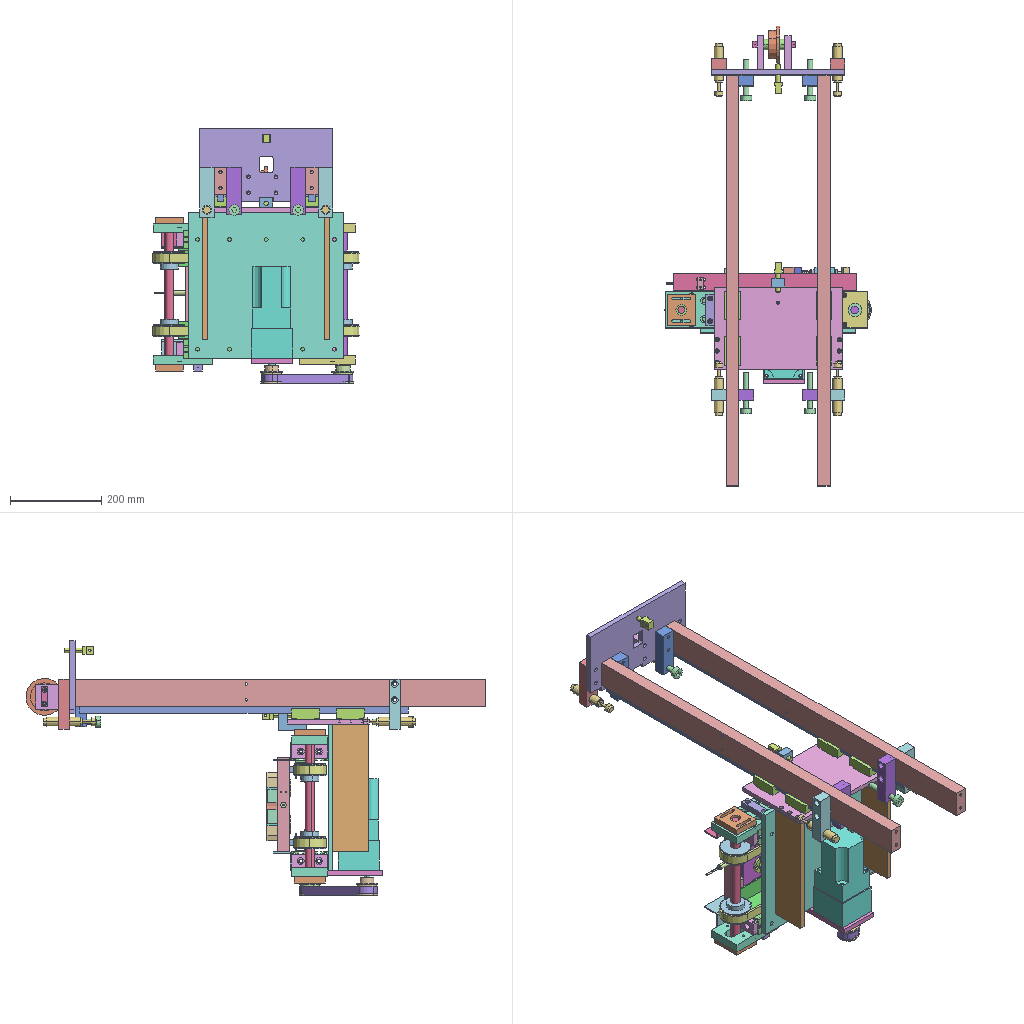Assembly | STEP file | 58 different items | 107 placed | box 451 x 1007 x 558 mm
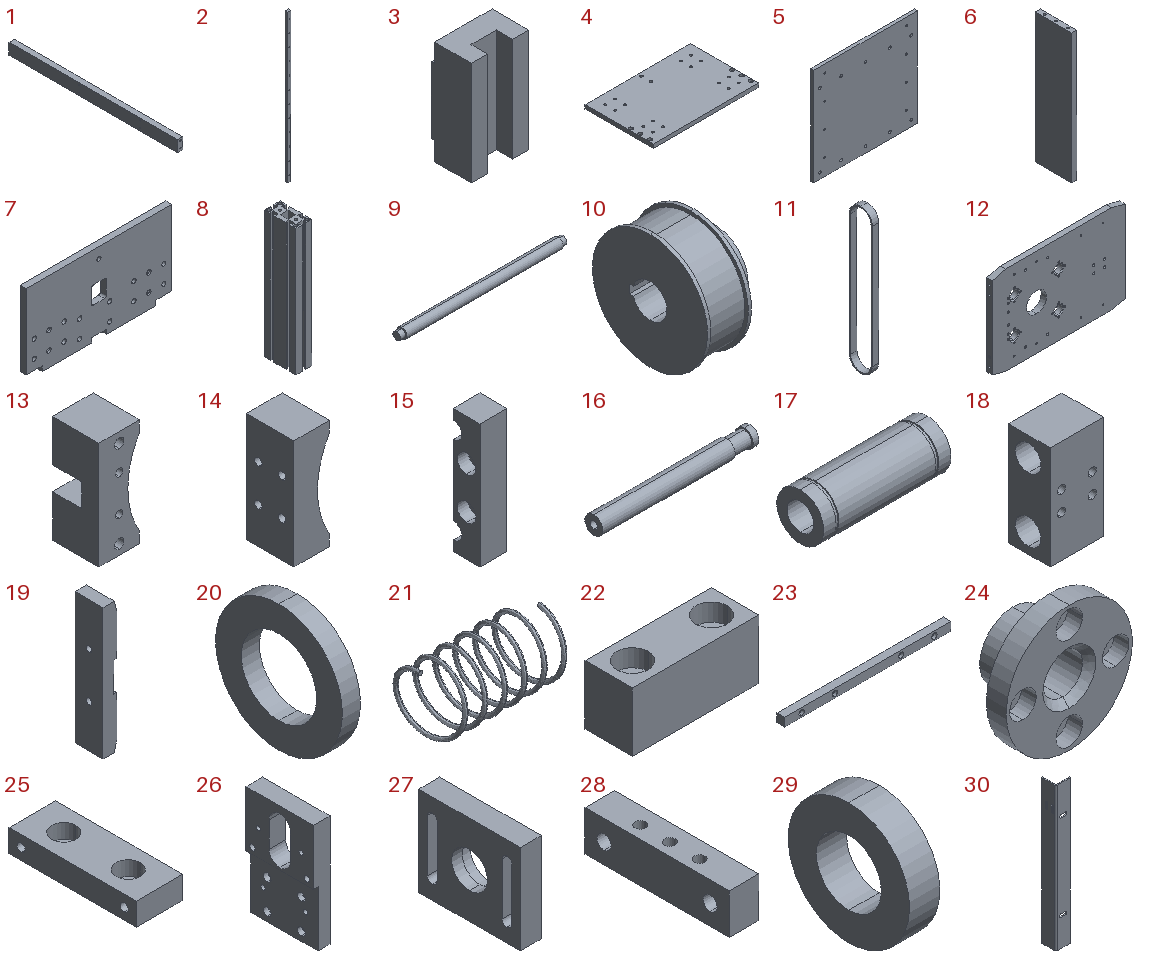Parts list (item | name | quantity | parent item | size | volume):
1 | PN_0061 (guide rail fixed plate) | x2 | - | 28 x 900 x 60 mm | 1504828 mm3
2 | PN_0027 (HGH15CA guide rail) | x2 | - | 15 x 14 x 720 mm | 146714 mm3
3 | PN_0017 (HGH15CA slider) | x4 | - | 34 x 23.7 x 61.4 mm | 38690 mm3
4 | PN_0009 (connecting block) | x1 | - | 280 x 180 x 10 mm | 491440 mm3
5 | PN_0064 (support block) | x1 | - | 340 x 10 x 320 mm | 1077927 mm3
6 | PN_0016 (inclined block) | x2 | - | 11 x 79 x 280 mm | 242077 mm3
7 | PN_0018 (fixed block) | x1 | - | 292 x 12 x 160 mm | 521488 mm3
8 | PN_0045 (cross beam) | x2 | - | 40 x 80 x 320 mm | 588947 mm3
9 | PN_0041 (follower wheel) | x1 | - | 328 x 20 x 20 mm | 99023 mm3
10 | PN_0051 (wheel) | x4 | - | 38 x 68 x 68 mm | 87974 mm3
11 | PN_0023 (conveyor belt) | x2 | - | 20 x 72 x 452 mm | 77890 mm3
12 | PN_0007 (tooling plate) | x1 | in PN_0025 (tooling assembly, return stroke) | 300 x 12 x 200 mm | 673943 mm3
13 | PN_0047 (semicircular tube block) | x1 | in PN_0025 (tooling assembly, return stroke) | 28 x 32 x 74 mm | 45440 mm3
14 | PN_0003 (movable semicircular tube block) | x1 | in PN_0025 (spring press assembly) | 24 x 32 x 74 mm | 45434 mm3
15 | PN_0010 (clamp block) | x2 | in PN_0025 (spring press assembly) | 16 x 16 x 74 mm | 15676 mm3
16 | PN_0040 (guide post) | x2 | in PN_0025 (spring press assembly) | 105 x 12 x 12 mm | 11156 mm3
17 | PN_0043 (linear bearing LM12LUU) | x2 | in PN_0025 (spring press assembly) | 57 x 21 x 21 mm | 13212 mm3
18 | PN_0008 (guide bushing seat) | x1 | in PN_0025 (spring press assembly) | 43.4 x 34 x 84 mm | 87676 mm3
19 | PN_0036 (connecting plate) | x1 | in PN_0025 (spring press assembly) | 16 x 32 x 150 mm | 73689 mm3
20 | PN_0033 (stop plate) | x2 | in PN_0025 (spring press assembly) | 3 x 21 x 21 mm | 670.926 mm3
21 | PN_0034 (spring) | x2 | in PN_0025 (spring press assembly) | 31 x 16 x 16 mm | 222.275 mm3
22 | PN_0035 (elastic pad) | x2 | in PN_0025 (tooling assembly, return stroke) | 32 x 12 x 15 mm | 4980 mm3
23 | PN_0013 (guide bar) | x2 | in PN_0025 (tooling assembly, return stroke) | 250 x 12 x 12.5 mm | 36132 mm3
24 | PN_0053 (guide bushing) | x4 | in PN_0025 (tooling assembly, return stroke) | 38 x 17 x 38 mm | 7268 mm3
25 | PN_0012 (reinforcing block) | x4 | - | 29 x 79 x 14 mm | 27118 mm3
26 | PN_0031 (connecting plate) | x2 | in PN_0002 (end seat assembly) | 19.5 x 79 x 130 mm | 136895 mm3
27 | PN_0052 (follower seat) | x2 | in PN_0002 (end seat assembly) | 14 x 68 x 60 mm | 42344 mm3
28 | PN_0019 (fixed plate) | x2 | in PN_0002 (end seat assembly) | 14 x 68 x 19 mm | 15184 mm3
29 | PN_0050 (ZZ6902) | x2 | in PN_0002 (end seat assembly) | 7 x 28 x 28 mm | 3073 mm3
30 | PN_0062 (side flange plate) | x1 | - | 40 x 40 x 400 mm | 89658 mm3
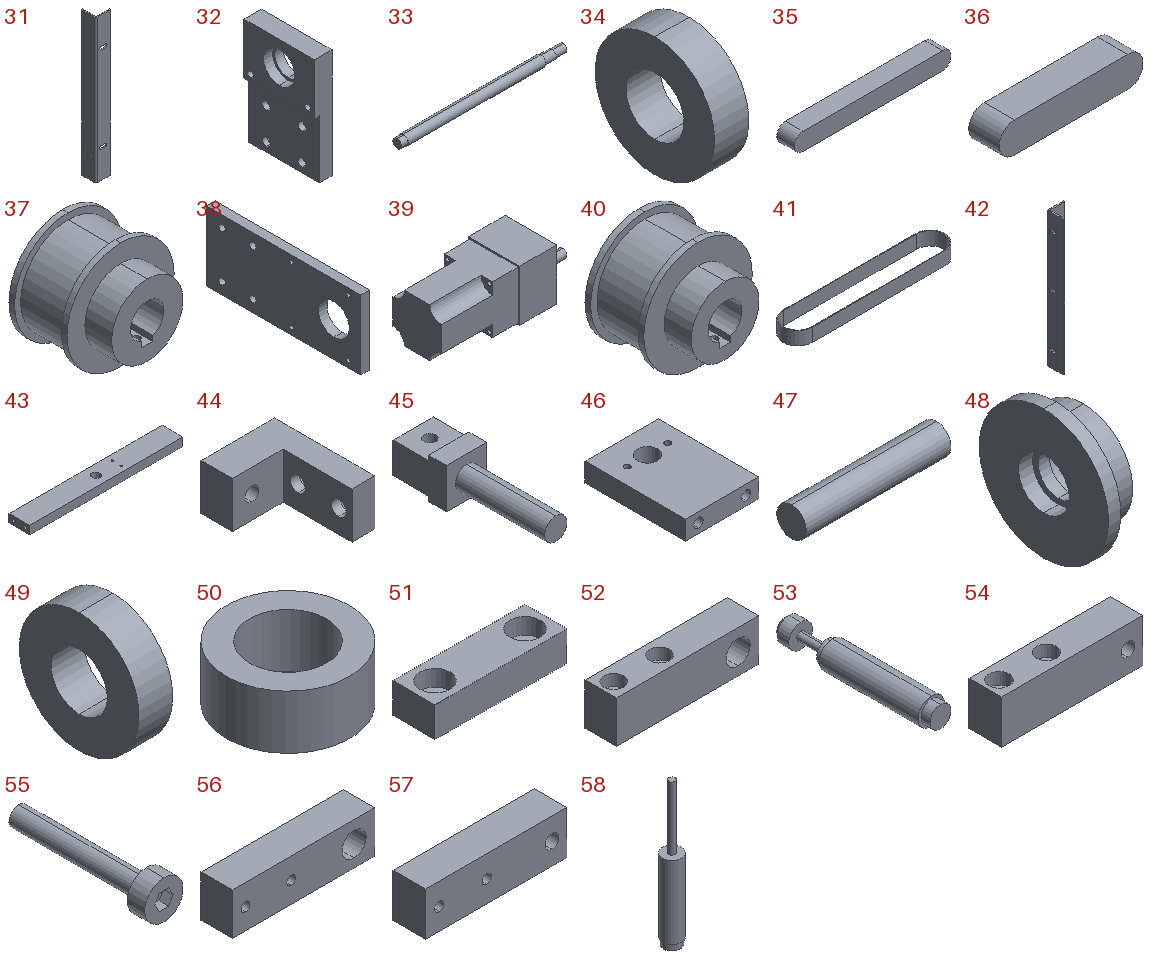31 | PN_0014 (side flange plate) | x1 | - | 40 x 40 x 400 mm | 89658 mm3
32 | PN_0042 (connecting plate) | x2 | - | 19.5 x 79 x 122 mm | 133748 mm3
33 | PN_0021 (drive wheel) | x1 | - | 325 x 20 x 20 mm | 94666 mm3
34 | PN_0044 (ZZ6003) | x2 | - | 10 x 35 x 35 mm | 7351 mm3
35 | PN_0039 (key 5x5x40) | x4 | - | 45 x 5 x 5 mm | 1098 mm3
36 | PN_0029 (key 4x4x15) | x1 | - | 19 x 4 x 4 mm | 290.265 mm3
37 | PN_0005 (ATP14L075)_ATP22XL050-A-H8 | x1 | - | 48 x 38 x 48 mm | 41242 mm3
38 | PN_0001 (motor mounting plate) | x1 | in PN_0002 (motor assembly) | 11 x 200 x 90 mm | 180816 mm3
39 | PN_0032 (60W.1: 15) | x1 | in PN_0002 (motor assembly) | 238 x 90 x 90 mm | 1379919 mm3
40 | PN_0006 (ATP14L075)_ATP22XL050-A-H8 | x1 | in PN_0002 (motor assembly) | 48 x 38 x 48 mm | 40082 mm3
41 | PN_0020 (timing belt 210L, width 20, Z=56) | x1 | - | 244.45 x 44.45 x 20 mm | 10730 mm3
42 | PN_0037 (belt clamp block) | x2 | - | 40 x 40 x 340 mm | 77417 mm3
43 | PN_0060 (stop block) | x1 | - | 206 x 28 x 11 mm | 61677 mm3
44 | PN_0063 (connecting block) | x1 | - | 45 x 61 x 28 mm | 35599 mm3
45 | PN_0055 (hook) | x2 | - | 18 x 64 x 18 mm | 9415 mm3
46 | PN_0046 (support block) | x2 | in PN_0002 (transition wheel assembly) | 54 x 74 x 14 mm | 51598 mm3
47 | PN_0054 (roller post) | x1 | in PN_0002 (transition wheel assembly) | 74 x 15 x 15 mm | 13077 mm3
48 | PN_0026 (sprocket z=16,p=15.875) | x1 | in PN_0002 (sprocket) | 25 x 81.37 x 81.37 mm | 74577 mm3
49 | PN_0057 (ZZ6002) | x2 | in PN_0002 (sprocket) | 9 x 32 x 32 mm | 5648 mm3
50 | PN_0059 (stop plate) | x2 | in PN_0002 (transition wheel assembly) | 24 x 24 x 10.5 mm | 2895 mm3
51 | PN_0056 (stop block) | x2 | in PN_0002 (transition wheel assembly) | 44 x 14 x 10 mm | 5093 mm3
52 | PN_0030 (buffer fixed block) | x2 | in PN_0002 (lower buffer assembly) | 109 x 24 x 32 mm | 69208 mm3
53 | PN_0058 (hydraulic buffer ACA2020) | x4 | in PN_0002 (lower buffer assembly), PN_0002 (upper buffer assembly) | 20 x 118 x 20 mm | 29167 mm3
54 | PN_0049 (locating fixed block) | x2 | in PN_0002 (lower locating assembly) | 104 x 24 x 32 mm | 69858 mm3
55 | PN_0028 (M12X60) | x4 | in PN_0002 (lower locating assembly), PN_0002 (upper locating assembly) | 24 x 91 x 24 mm | 13504 mm3
56 | PN_0024 (buffer fixed block) | x2 | in PN_0002 (upper buffer assembly) | 109 x 24 x 32 mm | 75518 mm3
57 | PN_0048 (locating fixed block) | x2 | in PN_0002 (upper locating assembly) | 104 x 24 x 32 mm | 76168 mm3
58 | PN_0022 (M12-4 proximity switch) | x1 | - | 12 x 12 x 90 mm | 6055 mm3
Placements (level | parent | child | x y z in mm | rotation matrix by rows):
1 | subassembly 2 | PN_0061 (guide rail fixed plate) | -56.042 -205.053 -30.0 | 1 0 0 0 1 0 0 0 1
1 | subassembly 2 | PN_0027 (HGH15CA guide rail) | -56.042 684.947 -30.0 | 1 0 0 0 0 1 0 -1 0
1 | subassembly 2 | PN_0017 (HGH15CA slider) | -56.042 90.647 -34.3 | 1 0 0 0 0 1 0 -1 -0
1 | subassembly 2 | PN_0061 (guide rail fixed plate) | 143.958 -205.053 -30.0 | 1 0 0 0 1 0 0 0 1
1 | subassembly 2 | PN_0027 (HGH15CA guide rail) | 143.958 684.947 -30.0 | 1 0 0 0 0 1 0 -1 0
1 | subassembly 2 | PN_0017 (HGH15CA slider) | 143.958 90.647 -34.3 | 1 0 0 0 0 1 0 -1 -0
1 | subassembly 2 | PN_0009 (connecting block) | 43.958 140.647 -68.0 | 1 0 0 0 1 0 0 0 1
1 | subassembly 2 | PN_0064 (support block) | 43.958 130.647 -68.0 | 1 0 0 0 1 0 0 0 1
1 | subassembly 2 | PN_0016 (inclined block) | 177.958 51.647 -68.0 | 1 0 0 0 1 0 0 0 1
1 | subassembly 2 | PN_0016 (inclined block) | -90.042 51.647 -68.0 | 1 0 0 0 1 0 0 0 1
1 | subassembly 2 | PN_0018 (fixed block) | 43.958 694.947 -45.0 | 1 0 0 0 1 0 0 0 1
1 | subassembly 2 | subassembly 3 | -18.042 169.332 -81.67 | 0 0 -1 0 1 0 1 0 -0
2 | subassembly 3 | PN_0045 (cross beam) | -46.33 11.315 -200.0 | 1 0 0 0 1 0 0 0 1
2 | subassembly 3 | PN_0045 (cross beam) | -286.33 11.315 -200.0 | 1 0 0 0 1 0 0 0 1
2 | subassembly 3 | PN_0041 (follower wheel) | -330.33 11.315 150.0 | 1 0 0 0 0.9618 -0.2738 0 0.2738 0.9618
2 | subassembly 3 | PN_0051 (wheel) | -73.33 11.315 150.0 | -1 0 0 0 0.9618 0.2738 0 0.2738 -0.9618
2 | subassembly 3 | PN_0023 (conveyor belt) | -86.33 11.315 150.0 | -1 0 0 0 -1 0 0 0 1
2 | subassembly 3 | PN_0051 (wheel) | -259.33 11.315 150.0 | 1 0 0 0 0.9618 -0.2738 0 0.2738 0.9618
2 | subassembly 3 | PN_0023 (conveyor belt) | -246.33 11.315 150.0 | -1 0 0 0 -1 0 0 0 1
2 | subassembly 3 | PN_0025 (tooling assembly, return stroke) | -166.33 74.53 -98.044 | 0 0 1 0 1 0 -1 0 -0
3 | PN_0025 (tooling assembly, return stroke) | PN_0007 (tooling plate) | -75.335 -9.216 -0.0 | 1 0 0 0 1 0 0 0 1
3 | PN_0025 (tooling assembly, return stroke) | PN_0047 (semicircular tube block) | -153.335 12.784 -0.0 | 1 0 0 0 1 0 0 0 1
3 | PN_0025 (tooling assembly, return stroke) | PN_0025 (spring press assembly) | -58.515 11.875 -0.0 | -1 0 0 0 1 0 0 0 -1
4 | PN_0025 (spring press assembly) | PN_0003 (movable semicircular tube block) | -57.18 2.909 -0.0 | 1 0 0 0 1 0 0 0 1
4 | PN_0025 (spring press assembly) | PN_0010 (clamp block) | -73.18 -13.091 -0.0 | 1 0 0 0 1 0 0 0 1
4 | PN_0025 (spring press assembly) | PN_0010 (clamp block) | -73.18 18.909 -0.0 | 1 0 0 0 -1 0 0 0 -1
4 | PN_0025 (spring press assembly) | PN_0040 (guide post) | -162.18 2.909 -26.0 | 1 0 0 0 0.9992 -0.03879 0 0.03879 0.9992
4 | PN_0025 (spring press assembly) | PN_0040 (guide post) | -162.18 2.909 26.0 | 1 0 0 0 0.4218 -0.9067 0 0.9067 0.4218
4 | PN_0025 (spring press assembly) | PN_0043 (linear bearing LM12LUU) | -153.18 2.909 -26.0 | 1 0 0 0 1 0 0 0 1
4 | PN_0025 (spring press assembly) | PN_0043 (linear bearing LM12LUU) | -153.18 2.909 26.0 | 1 0 0 0 1 0 0 0 1
4 | PN_0025 (spring press assembly) | PN_0008 (guide bushing seat) | -124.68 -15.091 -0.0 | 1 0 0 0 1 0 0 0 1
4 | PN_0025 (spring press assembly) | PN_0036 (connecting plate) | -178.18 2.909 -0.0 | 1 0 0 0 1 0 0 0 1
4 | PN_0025 (spring press assembly) | PN_0033 (stop plate) | -96.18 2.909 26.0 | 1 0 0 0 1 0 0 0 1
4 | PN_0025 (spring press assembly) | PN_0033 (stop plate) | -96.18 2.909 -26.0 | 1 0 0 0 1 0 0 0 1
4 | PN_0025 (spring press assembly) | PN_0034 (spring) | -97.732 2.909 26.0 | 1 0 0 0 1 0 0 0 1
4 | PN_0025 (spring press assembly) | PN_0034 (spring) | -97.081 2.909 -26.0 | 1 0 0 0 0.9742 -0.2257 0 0.2257 0.9742
3 | PN_0025 (tooling assembly, return stroke) | PN_0035 (elastic pad) | -175.335 -9.216 -70.0 | 0 0 -1 0 1 0 1 0 0
3 | PN_0025 (tooling assembly, return stroke) | PN_0035 (elastic pad) | -175.335 -9.216 70.0 | 0 0 -1 0 1 0 1 0 0
3 | PN_0025 (tooling assembly, return stroke) | PN_0013 (guide bar) | -25.335 -27.215 80.0 | 1 0 0 0 1 0 0 0 1
3 | PN_0025 (tooling assembly, return stroke) | PN_0013 (guide bar) | -25.335 -27.215 -80.0 | 1 0 0 0 1 0 0 0 1
3 | PN_0025 (tooling assembly, return stroke) | PN_0053 (guide bushing) | -125.335 -21.215 40.0 | 1 0 0 0 1 0 0 0 1
3 | PN_0025 (tooling assembly, return stroke) | PN_0053 (guide bushing) | -125.335 -21.215 -40.0 | 1 0 0 0 1 0 0 0 1
3 | PN_0025 (tooling assembly, return stroke) | PN_0053 (guide bushing) | -25.335 -21.215 40.0 | 1 0 0 0 1 0 0 0 1
3 | PN_0025 (tooling assembly, return stroke) | PN_0053 (guide bushing) | -25.335 -21.215 -40.0 | 1 0 0 0 1 0 0 0 1
2 | subassembly 3 | PN_0012 (reinforcing block) | -46.33 11.315 120.0 | 1 0 0 0 1 0 0 0 1
2 | subassembly 3 | PN_0012 (reinforcing block) | -286.33 11.315 120.0 | 1 0 0 0 1 0 0 0 1
2 | subassembly 3 | PN_0012 (reinforcing block) | -46.33 11.315 -200.0 | -1 0 0 0 1 0 0 0 -1
2 | subassembly 3 | PN_0012 (reinforcing block) | -286.33 11.315 -200.0 | -1 0 0 0 1 0 0 0 -1
2 | subassembly 3 | PN_0002 (end seat assembly) | -332.66 22.63 -80.0 | -1 0 0 0 -1 0 0 0 1
3 | PN_0002 (end seat assembly) | PN_0031 (connecting plate) | -31.83 11.315 135.0 | 1 0 0 0 1 0 0 0 1
3 | PN_0002 (end seat assembly) | PN_0052 (follower seat) | -5.33 11.315 230.0 | -1 0 0 0 1 0 0 0 -1
3 | PN_0002 (end seat assembly) | PN_0019 (fixed plate) | -5.33 11.315 167.0 | 1 0 0 0 1 0 0 0 1
3 | PN_0002 (end seat assembly) | PN_0050 (ZZ6902) | -12.33 11.315 230.0 | 1 0 0 0 1 0 0 0 1
2 | subassembly 3 | PN_0002 (end seat assembly) | -0.0 -0.0 -80.0 | 1 0 0 0 1 0 0 0 1
3 | PN_0002 (end seat assembly) | PN_0031 (connecting plate) | -31.83 11.315 135.0 | 1 0 0 0 1 0 0 0 1
3 | PN_0002 (end seat assembly) | PN_0052 (follower seat) | -5.33 11.315 230.0 | -1 0 0 0 1 0 0 0 -1
3 | PN_0002 (end seat assembly) | PN_0019 (fixed plate) | -5.33 11.315 167.0 | 1 0 0 0 1 0 0 0 1
3 | PN_0002 (end seat assembly) | PN_0050 (ZZ6902) | -12.33 11.315 230.0 | 1 0 0 0 1 0 0 0 1
2 | subassembly 3 | PN_0062 (side flange plate) | -66.33 51.315 167.248 | 1 0 0 0 1 0 0 0 1
2 | subassembly 3 | PN_0014 (side flange plate) | -266.33 51.315 -233.53 | -1 0 0 0 1 0 0 0 -1
2 | subassembly 3 | PN_0042 (connecting plate) | -31.83 11.315 -135.0 | 1 0 0 0 -1 0 0 0 -1
2 | subassembly 3 | PN_0042 (connecting plate) | -300.83 11.315 -135.0 | -1 0 0 0 1 0 0 0 -1
2 | subassembly 3 | PN_0021 (drive wheel) | -19.83 11.315 -230.0 | -1 0 0 0 0.9997 0.02567 0 0.02567 -0.9997
2 | subassembly 3 | PN_0044 (ZZ6003) | -310.83 11.315 -230.0 | 1 0 0 0 1 0 0 0 1
2 | subassembly 3 | PN_0044 (ZZ6003) | -31.83 11.315 -230.0 | 1 0 0 0 1 0 0 0 1
2 | subassembly 3 | PN_0039 (key 5x5x40) | -240.33 18.047 151.917 | 1 0 0 0 0.9618 -0.2738 0 0.2738 0.9618
2 | subassembly 3 | PN_0039 (key 5x5x40) | -92.33 18.047 151.917 | 1 0 0 0 0.9618 -0.2738 0 0.2738 0.9618
2 | subassembly 3 | PN_0039 (key 5x5x40) | -240.33 18.313 -229.82 | 1 0 0 0 0.9997 -0.02567 0 0.02567 0.9997
2 | subassembly 3 | PN_0039 (key 5x5x40) | -92.33 18.313 -229.82 | 1 0 0 0 0.9997 -0.02567 0 0.02567 0.9997
2 | subassembly 3 | PN_0051 (wheel) | -73.33 11.315 -230.0 | -1 0 0 0 0.9997 0.02567 0 0.02567 -0.9997
2 | subassembly 3 | PN_0051 (wheel) | -259.33 11.315 -230.0 | 1 0 0 0 0.9997 -0.02567 0 0.02567 0.9997
2 | subassembly 3 | PN_0029 (key 4x4x15) | -333.33 16.313 -229.872 | 1 0 0 0 0.9997 -0.02567 0 0.02567 0.9997
2 | subassembly 3 | PN_0005 (ATP14L075)_ATP22XL050-A-H8 | -337.33 11.315 -230.0 | 0 -1 0 0.9317 0 -0.3631 0.3631 0 0.9317
2 | subassembly 3 | PN_0002 (motor assembly) | -349.597 -58.379 -73.875 | -1 0 0 0 1 0 0 0 -1
3 | PN_0002 (motor assembly) | PN_0001 (motor mounting plate) | -37.767 -90.306 0.0 | 1 0 0 0 1 0 0 0 1
3 | PN_0002 (motor assembly) | PN_0032 (60W.1: 15) | -108.267 -37.306 0.0 | 1 0 0 0 1 0 0 0 1
3 | PN_0002 (motor assembly) | PN_0006 (ATP14L075)_ATP22XL050-A-H8 | -12.267 -55.306 0.0 | 0 1 0 -0.1427 0 -0.9898 -0.9898 0 0.1427
2 | subassembly 3 | PN_0020 (timing belt 210L, width 20, Z=56) | -351.58 -51.185 -151.938 | 0 0 1 0.625 0.7806 0 -0.7806 0.625 0
2 | subassembly 3 | PN_0037 (belt clamp block) | -266.33 3.315 130.0 | 1 0 0 0 1 0 0 0 1
2 | subassembly 3 | PN_0037 (belt clamp block) | -66.33 3.315 -210.0 | -1 0 0 0 1 0 0 0 -1
2 | subassembly 3 | PN_0060 (stop block) | -163.33 55.315 108.089 | 1 0 0 0 1 0 0 0 1
1 | subassembly 2 | PN_0017 (HGH15CA slider) | -56.042 190.647 -34.3 | 1 0 0 0 0 1 0 -1 -0
1 | subassembly 2 | PN_0017 (HGH15CA slider) | 143.958 190.647 -34.3 | 1 0 0 0 0 1 0 -1 -0
1 | subassembly 2 | PN_0063 (connecting block) | 43.958 188.647 -82.0 | 0 0 1 0 1 0 -1 0 0
1 | subassembly 2 | PN_0055 (hook) | 43.958 220.647 -49.0 | 0 0 1 0 1 0 -1 0 0
1 | subassembly 2 | PN_0002 (transition wheel assembly) | 5.358 752.51 1.624 | 0 0 -1 0 1 0 1 0 0
2 | PN_0002 (transition wheel assembly) | PN_0046 (support block) | -9.939 -45.563 -0.0 | 1 0 0 0 1 0 0 0 1
2 | PN_0002 (transition wheel assembly) | PN_0046 (support block) | -9.939 -45.563 -60.0 | 1 0 0 0 1 0 0 0 1
2 | PN_0002 (transition wheel assembly) | PN_0054 (roller post) | -9.939 9.437 -30.0 | 0 -0.03289 0.9995 0 0.9995 0.03289 -1 0 0
2 | PN_0002 (transition wheel assembly) | PN_0002 (sprocket) | -9.323 17.636 -38.04 | 0 0.07491 -0.9972 0 0.9972 0.07491 1 0 0
3 | PN_0002 (sprocket) | PN_0026 (sprocket z=16,p=15.875) | -4.46 -8.221 0.0 | 1 0 0 0 0.8869 -0.4619 0 0.4619 0.8869
3 | PN_0002 (sprocket) | PN_0057 (ZZ6002) | 11.54 -8.221 -0.0 | 1 0 0 0 1 0 0 0 1
3 | PN_0002 (sprocket) | PN_0057 (ZZ6002) | -4.46 -8.221 -0.0 | 1 0 0 0 1 0 0 0 1
2 | PN_0002 (transition wheel assembly) | PN_0059 (stop plate) | -9.939 9.437 -17.5 | 1 0 0 0 1 0 0 0 1
2 | PN_0002 (transition wheel assembly) | PN_0059 (stop plate) | -9.939 9.437 -53.0 | 0.9993 0.03637 0 -0.03637 0.9993 0 0 0 1
2 | PN_0002 (transition wheel assembly) | PN_0056 (stop block) | -9.939 9.437 7.0 | 1 0 0 0 1 0 0 0 1
2 | PN_0002 (transition wheel assembly) | PN_0056 (stop block) | -9.939 9.437 -67.0 | -1 0 0 0 1 0 0 0 -1
1 | subassembly 2 | PN_0055 (hook) | 43.958 718.947 93.5 | 0 0 -1 0 -1 0 -1 0 0
1 | subassembly 2 | PN_0002 (lower buffer assembly) | 173.958 -10.863 -72.058 | 0 0 1 0 1 0 -1 0 0
2 | PN_0002 (lower buffer assembly) | PN_0030 (buffer fixed block) | -102.058 5.81 -0.0 | 1 0 0 0 1 0 0 0 1
2 | PN_0002 (lower buffer assembly) | PN_0058 (hydraulic buffer ACA2020) | -9.058 -40.34 -0.0 | 1 0 0 0 1 0 0 0 1
1 | subassembly 2 | PN_0002 (lower buffer assembly) | -86.042 -10.863 -72.058 | 0 0 1 0 1 0 -1 0 0
2 | PN_0002 (lower buffer assembly) | PN_0030 (buffer fixed block) | -102.058 5.81 -0.0 | 1 0 0 0 1 0 0 0 1
2 | PN_0002 (lower buffer assembly) | PN_0058 (hydraulic buffer ACA2020) | -9.058 -40.34 -0.0 | 1 0 0 0 1 0 0 0 1
1 | subassembly 2 | PN_0002 (lower locating assembly) | -26.042 -3.218 -34.749 | 0 0 -1 0 -1 0 -1 0 0
2 | PN_0002 (lower locating assembly) | PN_0049 (locating fixed block) | -64.749 1.835 -0.0 | 1 0 0 0 1 0 0 0 1
2 | PN_0002 (lower locating assembly) | PN_0028 (M12X60) | 28.251 43.274 0.0 | -0.9457 0 0.3251 0 -1 0 0.3251 0 0.9457
1 | subassembly 2 | PN_0002 (lower locating assembly) | 113.958 -3.218 -34.749 | 0 0 -1 0 -1 0 -1 0 0
2 | PN_0002 (lower locating assembly) | PN_0049 (locating fixed block) | -64.749 1.835 -0.0 | 1 0 0 0 1 0 0 0 1
2 | PN_0002 (lower locating assembly) | PN_0028 (M12X60) | 28.251 43.274 0.0 | -0.9457 0 0.3251 0 -1 0 0.3251 0 0.9457
1 | subassembly 2 | PN_0002 (upper buffer assembly) | 173.958 724.757 -72.058 | 0 0 -1 0 -1 0 -1 0 -0
2 | PN_0002 (upper buffer assembly) | PN_0024 (buffer fixed block) | -102.058 5.81 0.0 | 1 0 0 0 1 0 0 0 1
2 | PN_0002 (upper buffer assembly) | PN_0058 (hydraulic buffer ACA2020) | -9.058 -40.34 -0.0 | 1 0 0 0 1 0 0 0 1
1 | subassembly 2 | PN_0002 (upper buffer assembly) | -86.042 724.757 -72.058 | 0 0 -1 0 -1 0 -1 0 -0
2 | PN_0002 (upper buffer assembly) | PN_0024 (buffer fixed block) | -102.058 5.81 0.0 | 1 0 0 0 1 0 0 0 1
2 | PN_0002 (upper buffer assembly) | PN_0058 (hydraulic buffer ACA2020) | -9.058 -40.34 -0.0 | 1 0 0 0 1 0 0 0 1
1 | subassembly 2 | PN_0002 (upper locating assembly) | 113.958 681.112 -34.749 | 0 0 1 0 1 0 -1 0 -0
2 | PN_0002 (upper locating assembly) | PN_0048 (locating fixed block) | -64.749 1.835 0.0 | 1 0 0 0 1 0 0 0 1
2 | PN_0002 (upper locating assembly) | PN_0028 (M12X60) | 28.251 -42.058 0.0 | 0.9854 0 0.1701 0 1 0 -0.1701 0 0.9854
1 | subassembly 2 | PN_0002 (upper locating assembly) | -26.042 681.112 -34.749 | 0 0 1 0 1 0 -1 0 -0
2 | PN_0002 (upper locating assembly) | PN_0048 (locating fixed block) | -64.749 1.835 0.0 | 1 0 0 0 1 0 0 0 1
2 | PN_0002 (upper locating assembly) | PN_0028 (M12X60) | 28.251 -42.058 0.0 | 0.9854 0 0.1701 0 1 0 -0.1701 0 0.9854
1 | subassembly 2 | PN_0022 (M12-4 proximity switch) | -109.856 238.647 -245.0 | 0 0 -1 -0.3449 0.9386 0 0.9386 0.3449 -0